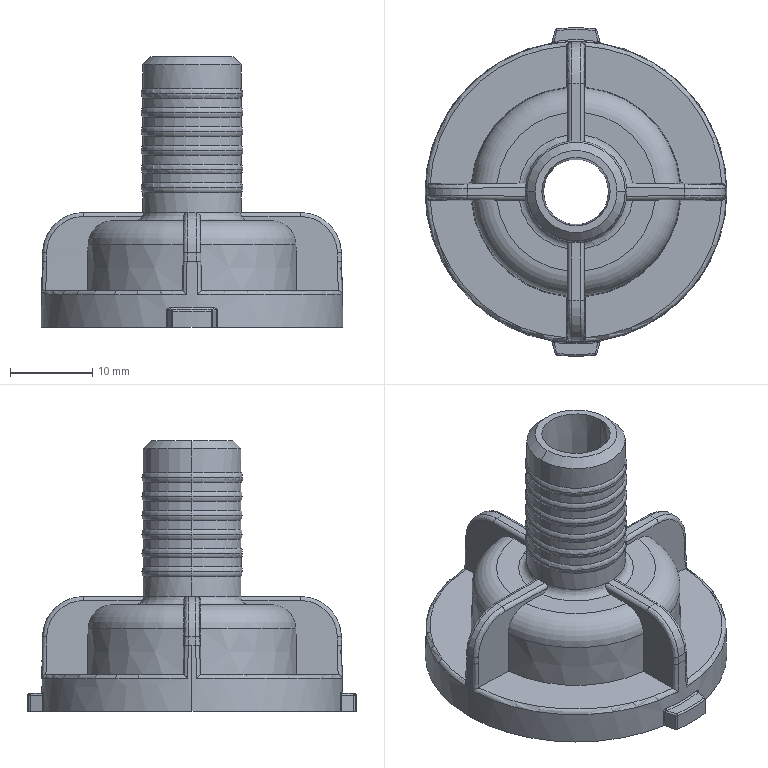Part | STEP file | ZXCOMPANY_A722-L-149 | 1 solid | 179 faces | box 36.755 x 40 x 33 mm | volume 6342 mm3 | torus 46 | cylinder 42 | plane 33 | spline 31 | cone 17 | other 6 | sphere 4 | commonest cylinder face diameters 12 x14 21.4 x10 0.4 x8 1 x8 40 x2